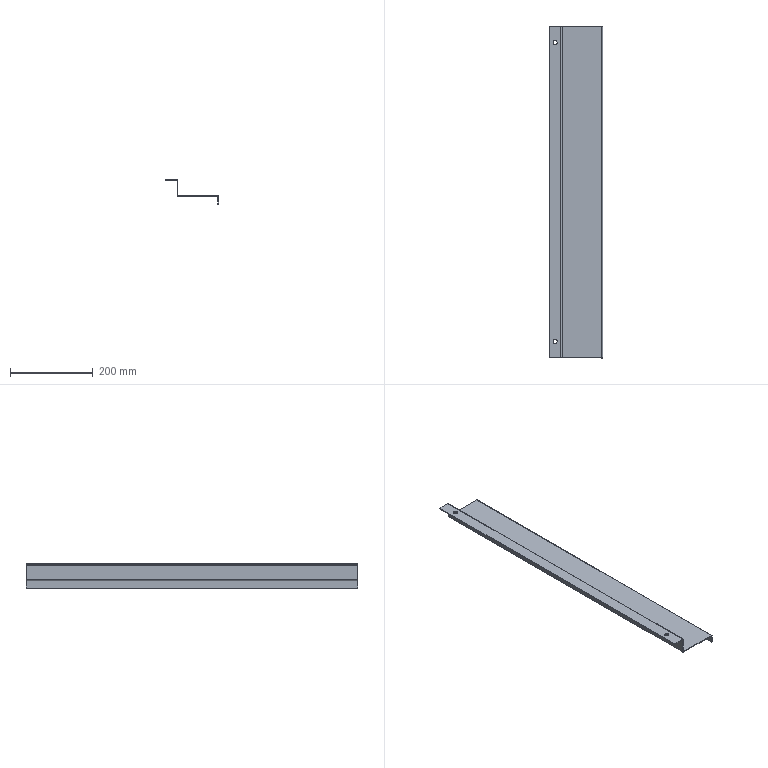Part | SolidWorks | features EdgeFlange 3, FlatPattern 1, ICE 1, SMBaseFlange 1, SheetMetal 1 | 1 solid | 34 faces | box 128 x 800 x 58 mm | volume 290508 mm3 | plane 24 | cylinder 10 | commonest cylinder face diameters 10 x4 1.473 x3 5.473 x3
STEP:
#1=CARTESIAN_POINT('',(-43.414,41.343,36.));
#2=VERTEX_POINT('',#1);
#3=CARTESIAN_POINT('',(-53.414,41.343,36.));
#4=VERTEX_POINT('',#3);
#5=CARTESIAN_POINT('',(-48.414,41.343,36.));
#6=DIRECTION('',(0.,0.,-1.));
#7=DIRECTION('',(-1.,0.,0.));
#8=AXIS2_PLACEMENT_3D('',#5,#6,#7);
#9=CIRCLE('',#8,5.);
#10=EDGE_CURVE('',#2,#4,#9,.T.);
#11=ORIENTED_EDGE('',*,*,#10,.T.);
#12=CARTESIAN_POINT('',(-53.414,41.343,38.));
#13=VERTEX_POINT('',#12);
#14=CARTESIAN_POINT('',(-53.414,41.343,28.));
#15=DIRECTION('',(0.,0.,1.));
#16=VECTOR('',#15,1000.);
#17=LINE('',#14,#16);
#18=EDGE_CURVE('',#4,#13,#17,.T.);
#19=ORIENTED_EDGE('',*,*,#18,.T.);
#20=CARTESIAN_POINT('',(-43.414,41.343,38.));
#21=VERTEX_POINT('',#20);
#22=CARTESIAN_POINT('',(-48.414,41.343,38.));
#23=DIRECTION('',(0.,0.,1.));
#24=DIRECTION('',(1.,0.,0.));
#25=AXIS2_PLACEMENT_3D('',#22,#23,#24);
#26=CIRCLE('',#25,5.);
#27=EDGE_CURVE('',#13,#21,#26,.T.);
#28=ORIENTED_EDGE('',*,*,#27,.T.);
#29=CARTESIAN_POINT('',(-43.414,41.343,28.));
#30=DIRECTION('',(0.,0.,1.));
#31=VECTOR('',#30,1000.);
#32=LINE('',#29,#31);
#33=EDGE_CURVE('',#2,#21,#32,.T.);
#34=ORIENTED_EDGE('',*,*,#33,.F.);
#35=EDGE_LOOP('',(#11,#19,#28,#34));
#36=FACE_OUTER_BOUND('',#35,.T.);
#37=CARTESIAN_POINT('',(-48.414,41.343,28.));
#38=DIRECTION('',(0.,0.,1.));
#39=DIRECTION('',(1.,0.,0.));
#40=AXIS2_PLACEMENT_3D('',#37,#38,#39);
#41=CYLINDRICAL_SURFACE('',#40,5.);
#42=ADVANCED_FACE('',(#36),#41,.F.);
#43=CARTESIAN_POINT('',(-43.414,-678.657,36.));
#44=VERTEX_POINT('',#43);
#45=CARTESIAN_POINT('',(-53.414,-678.657,36.));
#46=VERTEX_POINT('',#45);
#47=CARTESIAN_POINT('',(-48.414,-678.657,36.));
#48=DIRECTION('',(0.,0.,-1.));
#49=DIRECTION('',(-1.,0.,0.));
#50=AXIS2_PLACEMENT_3D('',#47,#48,#49);
#51=CIRCLE('',#50,5.);
#52=EDGE_CURVE('',#44,#46,#51,.T.);
#53=ORIENTED_EDGE('',*,*,#52,.T.);
#54=CARTESIAN_POINT('',(-53.414,-678.657,38.));
#55=VERTEX_POINT('',#54);
#56=CARTESIAN_POINT('',(-53.414,-678.657,28.));
#57=DIRECTION('',(0.,0.,1.));
#58=VECTOR('',#57,1000.);
#59=LINE('',#56,#58);
#60=EDGE_CURVE('',#46,#55,#59,.T.);
#61=ORIENTED_EDGE('',*,*,#60,.T.);
#62=CARTESIAN_POINT('',(-43.414,-678.657,38.));
#63=VERTEX_POINT('',#62);
#64=CARTESIAN_POINT('',(-48.414,-678.657,38.));
#65=DIRECTION('',(0.,0.,1.));
#66=DIRECTION('',(1.,0.,0.));
#67=AXIS2_PLACEMENT_3D('',#64,#65,#66);
#68=CIRCLE('',#67,5.);
#69=EDGE_CURVE('',#55,#63,#68,.T.);
#70=ORIENTED_EDGE('',*,*,#69,.T.);
#71=CARTESIAN_POINT('',(-43.414,-678.657,28.));
#72=DIRECTION('',(0.,0.,1.));
#73=VECTOR('',#72,1000.);
#74=LINE('',#71,#73);
#75=EDGE_CURVE('',#44,#63,#74,.T.);
#76=ORIENTED_EDGE('',*,*,#75,.F.);
#77=EDGE_LOOP('',(#53,#61,#70,#76));
#78=FACE_OUTER_BOUND('',#77,.T.);
#79=CARTESIAN_POINT('',(-48.414,-678.657,28.));
#80=DIRECTION('',(0.,0.,1.));
#81=DIRECTION('',(1.,0.,0.));
#82=AXIS2_PLACEMENT_3D('',#79,#80,#81);
#83=CYLINDRICAL_SURFACE('',#82,5.);
#84=ADVANCED_FACE('',(#78),#83,.F.);
#85=CARTESIAN_POINT('',(-34.046,-718.657,35.263));
#86=VERTEX_POINT('',#85);
#87=CARTESIAN_POINT('',(-32.046,-718.657,35.263));
#88=VERTEX_POINT('',#87);
#89=CARTESIAN_POINT('',(-34.046,-718.657,35.263));
#90=DIRECTION('',(1.,0.,0.));
#91=VECTOR('',#90,1000.);
#92=LINE('',#89,#91);
#93=EDGE_CURVE('',#86,#88,#92,.T.);
#94=ORIENTED_EDGE('',*,*,#93,.F.);
#95=CARTESIAN_POINT('',(-34.046,-718.657,0.7366));
#96=VERTEX_POINT('',#95);
#97=CARTESIAN_POINT('',(-34.046,-718.657,0.));
#98=DIRECTION('',(0.,0.,1.));
#99=VECTOR('',#98,1000.);
#100=LINE('',#97,#99);
#101=EDGE_CURVE('',#96,#86,#100,.T.);
#102=ORIENTED_EDGE('',*,*,#101,.F.);
#103=CARTESIAN_POINT('',(-32.046,-718.657,0.7366));
#104=VERTEX_POINT('',#103);
#105=CARTESIAN_POINT('',(-32.046,-718.657,0.7366));
#106=DIRECTION('',(-1.,0.,0.));
#107=VECTOR('',#106,1000.);
#108=LINE('',#105,#107);
#109=EDGE_CURVE('',#104,#96,#108,.T.);
#110=ORIENTED_EDGE('',*,*,#109,.F.);
#111=CARTESIAN_POINT('',(-32.046,-718.657,38.));
#112=DIRECTION('',(0.,0.,1.));
#113=VECTOR('',#112,1000.);
#114=LINE('',#111,#113);
#115=EDGE_CURVE('',#104,#88,#114,.T.);
#116=ORIENTED_EDGE('',*,*,#115,.T.);
#117=EDGE_LOOP('',(#94,#102,#110,#116));
#118=FACE_OUTER_BOUND('',#117,.T.);
#119=CARTESIAN_POINT('',(-34.046,-718.657,38.));
#120=DIRECTION('',(0.,1.,0.));
#121=DIRECTION('',(-1.,0.,0.));
#122=AXIS2_PLACEMENT_3D('',#119,#120,#121);
#123=PLANE('',#122);
#124=ADVANCED_FACE('',(#118),#123,.F.);
#125=CARTESIAN_POINT('',(-34.046,81.343,35.263));
#126=VERTEX_POINT('',#125);
#127=CARTESIAN_POINT('',(-32.046,81.343,35.263));
#128=VERTEX_POINT('',#127);
#129=CARTESIAN_POINT('',(-34.046,81.343,35.263));
#130=DIRECTION('',(1.,0.,0.));
#131=VECTOR('',#130,1000.);
#132=LINE('',#129,#131);
#133=EDGE_CURVE('',#126,#128,#132,.T.);
#134=ORIENTED_EDGE('',*,*,#133,.T.);
#135=CARTESIAN_POINT('',(-32.046,81.343,0.7366));
#136=VERTEX_POINT('',#135);
#137=CARTESIAN_POINT('',(-32.046,81.343,0.));
#138=DIRECTION('',(0.,0.,-1.));
#139=VECTOR('',#138,1000.);
#140=LINE('',#137,#139);
#141=EDGE_CURVE('',#128,#136,#140,.T.);
#142=ORIENTED_EDGE('',*,*,#141,.T.);
#143=CARTESIAN_POINT('',(-34.046,81.343,0.7366));
#144=VERTEX_POINT('',#143);
#145=CARTESIAN_POINT('',(-34.046,81.343,0.7366));
#146=DIRECTION('',(-1.,0.,0.));
#147=VECTOR('',#146,1000.);
#148=LINE('',#145,#147);
#149=EDGE_CURVE('',#136,#144,#148,.T.);
#150=ORIENTED_EDGE('',*,*,#149,.T.);
#151=CARTESIAN_POINT('',(-34.046,81.343,0.));
#152=DIRECTION('',(0.,0.,-1.));
#153=VECTOR('',#152,1000.);
#154=LINE('',#151,#153);
#155=EDGE_CURVE('',#126,#144,#154,.T.);
#156=ORIENTED_EDGE('',*,*,#155,.F.);
#157=EDGE_LOOP('',(#134,#142,#150,#156));
#158=FACE_OUTER_BOUND('',#157,.T.);
#159=CARTESIAN_POINT('',(-34.046,81.343,0.));
#160=DIRECTION('',(0.,-1.,0.));
#161=DIRECTION('',(0.,0.,-1.));
#162=AXIS2_PLACEMENT_3D('',#159,#160,#161);
#163=PLANE('',#162);
#164=ADVANCED_FACE('',(#158),#163,.F.);
#165=CARTESIAN_POINT('',(-34.046,81.343,35.263));
#166=DIRECTION('',(0.,-1.,0.));
#167=VECTOR('',#166,1000.);
#168=LINE('',#165,#167);
#169=EDGE_CURVE('',#126,#86,#168,.T.);
#170=ORIENTED_EDGE('',*,*,#169,.F.);
#171=ORIENTED_EDGE('',*,*,#155,.T.);
#172=CARTESIAN_POINT('',(-34.046,81.343,0.7366));
#173=DIRECTION('',(0.,1.,0.));
#174=VECTOR('',#173,1000.);
#175=LINE('',#172,#174);
#176=EDGE_CURVE('',#96,#144,#175,.T.);
#177=ORIENTED_EDGE('',*,*,#176,.F.);
#178=ORIENTED_EDGE('',*,*,#101,.T.);
#179=EDGE_LOOP('',(#170,#171,#177,#178));
#180=FACE_OUTER_BOUND('',#179,.T.);
#181=CARTESIAN_POINT('',(-34.046,0.,0.));
#182=DIRECTION('',(1.,0.,0.));
#183=DIRECTION('',(0.,0.,-1.));
#184=AXIS2_PLACEMENT_3D('',#181,#182,#183);
#185=PLANE('',#184);
#186=ADVANCED_FACE('',(#180),#185,.F.);
#187=ORIENTED_EDGE('',*,*,#141,.F.);
#188=CARTESIAN_POINT('',(-32.046,81.343,35.263));
#189=DIRECTION('',(0.,-1.,0.));
#190=VECTOR('',#189,1000.);
#191=LINE('',#188,#190);
#192=EDGE_CURVE('',#128,#88,#191,.T.);
#193=ORIENTED_EDGE('',*,*,#192,.T.);
#194=ORIENTED_EDGE('',*,*,#115,.F.);
#195=CARTESIAN_POINT('',(-32.046,81.343,0.7366));
#196=DIRECTION('',(0.,-1.,0.));
#197=VECTOR('',#196,1000.);
#198=LINE('',#195,#197);
#199=EDGE_CURVE('',#136,#104,#198,.T.);
#200=ORIENTED_EDGE('',*,*,#199,.F.);
#201=EDGE_LOOP('',(#187,#193,#194,#200));
#202=FACE_OUTER_BOUND('',#201,.T.);
#203=CARTESIAN_POINT('',(-32.046,0.,0.));
#204=DIRECTION('',(1.,0.,0.));
#205=DIRECTION('',(0.,0.,-1.));
#206=AXIS2_PLACEMENT_3D('',#203,#204,#205);
#207=PLANE('',#206);
#208=ADVANCED_FACE('',(#202),#207,.T.);
#209=CARTESIAN_POINT('',(-31.309,-718.657,-2.));
#210=VERTEX_POINT('',#209);
#211=CARTESIAN_POINT('',(63.218,-718.657,-2.));
#212=VERTEX_POINT('',#211);
#213=CARTESIAN_POINT('',(65.954,-718.657,-2.));
#214=DIRECTION('',(1.,0.,0.));
#215=VECTOR('',#214,1000.);
#216=LINE('',#213,#215);
#217=EDGE_CURVE('',#210,#212,#216,.T.);
#218=ORIENTED_EDGE('',*,*,#217,.T.);
#219=CARTESIAN_POINT('',(63.218,-718.657,0.));
#220=VERTEX_POINT('',#219);
#221=CARTESIAN_POINT('',(63.218,-718.657,-2.));
#222=DIRECTION('',(0.,0.,1.));
#223=VECTOR('',#222,1000.);
#224=LINE('',#221,#223);
#225=EDGE_CURVE('',#212,#220,#224,.T.);
#226=ORIENTED_EDGE('',*,*,#225,.T.);
#227=CARTESIAN_POINT('',(-31.309,-718.657,0.));
#228=VERTEX_POINT('',#227);
#229=CARTESIAN_POINT('',(65.954,-718.657,0.));
#230=DIRECTION('',(1.,0.,0.));
#231=VECTOR('',#230,1000.);
#232=LINE('',#229,#231);
#233=EDGE_CURVE('',#228,#220,#232,.T.);
#234=ORIENTED_EDGE('',*,*,#233,.F.);
#235=CARTESIAN_POINT('',(-31.309,-718.657,0.));
#236=DIRECTION('',(0.,0.,-1.));
#237=VECTOR('',#236,1000.);
#238=LINE('',#235,#237);
#239=EDGE_CURVE('',#228,#210,#238,.T.);
#240=ORIENTED_EDGE('',*,*,#239,.T.);
#241=EDGE_LOOP('',(#218,#226,#234,#240));
#242=FACE_OUTER_BOUND('',#241,.T.);
#243=CARTESIAN_POINT('',(65.954,-718.657,-2.));
#244=DIRECTION('',(0.,-1.,0.));
#245=DIRECTION('',(0.,0.,-1.));
#246=AXIS2_PLACEMENT_3D('',#243,#244,#245);
#247=PLANE('',#246);
#248=ADVANCED_FACE('',(#242),#247,.T.);
#249=CARTESIAN_POINT('',(63.218,81.343,-2.));
#250=VERTEX_POINT('',#249);
#251=CARTESIAN_POINT('',(-31.309,81.343,-2.));
#252=VERTEX_POINT('',#251);
#253=CARTESIAN_POINT('',(65.954,81.343,-2.));
#254=DIRECTION('',(-1.,0.,0.));
#255=VECTOR('',#254,1000.);
#256=LINE('',#253,#255);
#257=EDGE_CURVE('',#250,#252,#256,.T.);
#258=ORIENTED_EDGE('',*,*,#257,.F.);
#259=CARTESIAN_POINT('',(63.218,-718.657,-2.));
#260=DIRECTION('',(0.,1.,0.));
#261=VECTOR('',#260,1000.);
#262=LINE('',#259,#261);
#263=EDGE_CURVE('',#212,#250,#262,.T.);
#264=ORIENTED_EDGE('',*,*,#263,.F.);
#265=ORIENTED_EDGE('',*,*,#217,.F.);
#266=CARTESIAN_POINT('',(-31.309,-718.657,-2.));
#267=DIRECTION('',(0.,1.,0.));
#268=VECTOR('',#267,1000.);
#269=LINE('',#266,#268);
#270=EDGE_CURVE('',#210,#252,#269,.T.);
#271=ORIENTED_EDGE('',*,*,#270,.T.);
#272=EDGE_LOOP('',(#258,#264,#265,#271));
#273=FACE_OUTER_BOUND('',#272,.T.);
#274=CARTESIAN_POINT('',(0.,0.,-2.));
#275=DIRECTION('',(0.,0.,-1.));
#276=DIRECTION('',(-1.,0.,0.));
#277=AXIS2_PLACEMENT_3D('',#274,#275,#276);
#278=PLANE('',#277);
#279=ADVANCED_FACE('',(#273),#278,.T.);
#280=CARTESIAN_POINT('',(63.218,81.343,0.));
#281=VERTEX_POINT('',#280);
#282=CARTESIAN_POINT('',(63.218,-718.657,0.));
#283=DIRECTION('',(0.,1.,0.));
#284=VECTOR('',#283,1000.);
#285=LINE('',#282,#284);
#286=EDGE_CURVE('',#220,#281,#285,.T.);
#287=ORIENTED_EDGE('',*,*,#286,.T.);
#288=CARTESIAN_POINT('',(-31.309,81.343,0.));
#289=VERTEX_POINT('',#288);
#290=CARTESIAN_POINT('',(65.954,81.343,0.));
#291=DIRECTION('',(-1.,0.,0.));
#292=VECTOR('',#291,1000.);
#293=LINE('',#290,#292);
#294=EDGE_CURVE('',#281,#289,#293,.T.);
#295=ORIENTED_EDGE('',*,*,#294,.T.);
#296=CARTESIAN_POINT('',(-31.309,-718.657,0.));
#297=DIRECTION('',(0.,1.,0.));
#298=VECTOR('',#297,1000.);
#299=LINE('',#296,#298);
#300=EDGE_CURVE('',#228,#289,#299,.T.);
#301=ORIENTED_EDGE('',*,*,#300,.F.);
#302=ORIENTED_EDGE('',*,*,#233,.T.);
#303=EDGE_LOOP('',(#287,#295,#301,#302));
#304=FACE_OUTER_BOUND('',#303,.T.);
#305=CARTESIAN_POINT('',(0.,0.,0.));
#306=DIRECTION('',(0.,0.,-1.));
#307=DIRECTION('',(-1.,0.,0.));
#308=AXIS2_PLACEMENT_3D('',#305,#306,#307);
#309=PLANE('',#308);
#310=ADVANCED_FACE('',(#304),#309,.F.);
#311=CARTESIAN_POINT('',(63.218,81.343,-2.));
#312=DIRECTION('',(0.,0.,1.));
#313=VECTOR('',#312,1000.);
#314=LINE('',#311,#313);
#315=EDGE_CURVE('',#250,#281,#314,.T.);
#316=ORIENTED_EDGE('',*,*,#315,.F.);
#317=ORIENTED_EDGE('',*,*,#257,.T.);
#318=CARTESIAN_POINT('',(-31.309,81.343,0.));
#319=DIRECTION('',(0.,0.,-1.));
#320=VECTOR('',#319,1000.);
#321=LINE('',#318,#320);
#322=EDGE_CURVE('',#289,#252,#321,.T.);
#323=ORIENTED_EDGE('',*,*,#322,.F.);
#324=ORIENTED_EDGE('',*,*,#294,.F.);
#325=EDGE_LOOP('',(#316,#317,#323,#324));
#326=FACE_OUTER_BOUND('',#325,.T.);
#327=CARTESIAN_POINT('',(65.954,81.343,-2.));
#328=DIRECTION('',(0.,1.,0.));
#329=DIRECTION('',(-1.,0.,0.));
#330=AXIS2_PLACEMENT_3D('',#327,#328,#329);
#331=PLANE('',#330);
#332=ADVANCED_FACE('',(#326),#331,.T.);
#333=ORIENTED_EDGE('',*,*,#149,.F.);
#334=CARTESIAN_POINT('',(-31.309,81.343,0.7366));
#335=DIRECTION('',(0.,1.,0.));
#336=DIRECTION('',(0.,0.,-1.));
#337=AXIS2_PLACEMENT_3D('',#334,#335,#336);
#338=CIRCLE('',#337,0.7366);
#339=EDGE_CURVE('',#289,#136,#338,.T.);
#340=ORIENTED_EDGE('',*,*,#339,.F.);
#341=ORIENTED_EDGE('',*,*,#322,.T.);
#342=CARTESIAN_POINT('',(-31.309,81.343,0.7366));
#343=DIRECTION('',(0.,1.,0.));
#344=DIRECTION('',(0.,0.,-1.));
#345=AXIS2_PLACEMENT_3D('',#342,#343,#344);
#346=CIRCLE('',#345,2.737);
#347=EDGE_CURVE('',#252,#144,#346,.T.);
#348=ORIENTED_EDGE('',*,*,#347,.T.);
#349=EDGE_LOOP('',(#333,#340,#341,#348));
#350=FACE_OUTER_BOUND('',#349,.T.);
#351=CARTESIAN_POINT('',(-31.309,81.343,0.7366));
#352=DIRECTION('',(0.,1.,0.));
#353=DIRECTION('',(0.,0.,1.));
#354=AXIS2_PLACEMENT_3D('',#351,#352,#353);
#355=PLANE('',#354);
#356=ADVANCED_FACE('',(#350),#355,.T.);
#357=CARTESIAN_POINT('',(-31.309,-718.657,0.7366));
#358=DIRECTION('',(0.,-1.,0.));
#359=DIRECTION('',(0.,0.,-1.));
#360=AXIS2_PLACEMENT_3D('',#357,#358,#359);
#361=CIRCLE('',#360,0.7366);
#362=EDGE_CURVE('',#104,#228,#361,.T.);
#363=ORIENTED_EDGE('',*,*,#362,.F.);
#364=ORIENTED_EDGE('',*,*,#109,.T.);
#365=CARTESIAN_POINT('',(-31.309,-718.657,0.7366));
#366=DIRECTION('',(0.,-1.,0.));
#367=DIRECTION('',(0.,0.,-1.));
#368=AXIS2_PLACEMENT_3D('',#365,#366,#367);
#369=CIRCLE('',#368,2.737);
#370=EDGE_CURVE('',#96,#210,#369,.T.);
#371=ORIENTED_EDGE('',*,*,#370,.T.);
#372=ORIENTED_EDGE('',*,*,#239,.F.);
#373=EDGE_LOOP('',(#363,#364,#371,#372));
#374=FACE_OUTER_BOUND('',#373,.T.);
#375=CARTESIAN_POINT('',(-31.309,-718.657,0.7366));
#376=DIRECTION('',(0.,1.,0.));
#377=DIRECTION('',(0.,0.,1.));
#378=AXIS2_PLACEMENT_3D('',#375,#376,#377);
#379=PLANE('',#378);
#380=ADVANCED_FACE('',(#374),#379,.F.);
#381=ORIENTED_EDGE('',*,*,#270,.F.);
#382=ORIENTED_EDGE('',*,*,#370,.F.);
#383=ORIENTED_EDGE('',*,*,#176,.T.);
#384=ORIENTED_EDGE('',*,*,#347,.F.);
#385=EDGE_LOOP('',(#381,#382,#383,#384));
#386=FACE_OUTER_BOUND('',#385,.T.);
#387=CARTESIAN_POINT('',(-31.309,-718.657,0.7366));
#388=DIRECTION('',(0.,-1.,0.));
#389=DIRECTION('',(-1.,0.,0.));
#390=AXIS2_PLACEMENT_3D('',#387,#388,#389);
#391=CYLINDRICAL_SURFACE('',#390,2.737);
#392=ADVANCED_FACE('',(#386),#391,.T.);
#393=ORIENTED_EDGE('',*,*,#300,.T.);
#394=ORIENTED_EDGE('',*,*,#339,.T.);
#395=ORIENTED_EDGE('',*,*,#199,.T.);
#396=ORIENTED_EDGE('',*,*,#362,.T.);
#397=EDGE_LOOP('',(#393,#394,#395,#396));
#398=FACE_OUTER_BOUND('',#397,.T.);
#399=CARTESIAN_POINT('',(-31.309,-718.657,0.7366));
#400=DIRECTION('',(0.,-1.,0.));
#401=DIRECTION('',(-1.,0.,0.));
#402=AXIS2_PLACEMENT_3D('',#399,#400,#401);
#403=CYLINDRICAL_SURFACE('',#402,0.7366);
#404=ADVANCED_FACE('',(#398),#403,.F.);
#405=CARTESIAN_POINT('',(63.954,81.343,-2.737));
#406=VERTEX_POINT('',#405);
#407=CARTESIAN_POINT('',(65.954,81.343,-2.737));
#408=VERTEX_POINT('',#407);
#409=CARTESIAN_POINT('',(65.954,81.343,-2.737));
#410=DIRECTION('',(1.,0.,0.));
#411=VECTOR('',#410,1000.);
#412=LINE('',#409,#411);
#413=EDGE_CURVE('',#406,#408,#412,.T.);
#414=ORIENTED_EDGE('',*,*,#413,.F.);
#415=CARTESIAN_POINT('',(63.218,81.343,-2.737));
#416=DIRECTION('',(0.,1.,0.));
#417=DIRECTION('',(0.,0.,-1.));
#418=AXIS2_PLACEMENT_3D('',#415,#416,#417);
#419=CIRCLE('',#418,0.7366);
#420=EDGE_CURVE('',#250,#406,#419,.T.);
#421=ORIENTED_EDGE('',*,*,#420,.F.);
#422=ORIENTED_EDGE('',*,*,#315,.T.);
#423=CARTESIAN_POINT('',(63.218,81.343,-2.737));
#424=DIRECTION('',(0.,1.,0.));
#425=DIRECTION('',(0.,0.,-1.));
#426=AXIS2_PLACEMENT_3D('',#423,#424,#425);
#427=CIRCLE('',#426,2.737);
#428=EDGE_CURVE('',#281,#408,#427,.T.);
#429=ORIENTED_EDGE('',*,*,#428,.T.);
#430=EDGE_LOOP('',(#414,#421,#422,#429));
#431=FACE_OUTER_BOUND('',#430,.T.);
#432=CARTESIAN_POINT('',(63.218,81.343,-2.737));
#433=DIRECTION('',(0.,1.,0.));
#434=DIRECTION('',(0.,0.,1.));
#435=AXIS2_PLACEMENT_3D('',#432,#433,#434);
#436=PLANE('',#435);
#437=ADVANCED_FACE('',(#431),#436,.T.);
#438=CARTESIAN_POINT('',(63.954,-718.657,-2.737));
#439=VERTEX_POINT('',#438);
#440=CARTESIAN_POINT('',(63.218,-718.657,-2.737));
#441=DIRECTION('',(0.,-1.,0.));
#442=DIRECTION('',(0.,0.,-1.));
#443=AXIS2_PLACEMENT_3D('',#440,#441,#442);
#444=CIRCLE('',#443,0.7366);
#445=EDGE_CURVE('',#439,#212,#444,.T.);
#446=ORIENTED_EDGE('',*,*,#445,.F.);
#447=CARTESIAN_POINT('',(65.954,-718.657,-2.737));
#448=VERTEX_POINT('',#447);
#449=CARTESIAN_POINT('',(63.954,-718.657,-2.737));
#450=DIRECTION('',(1.,0.,0.));
#451=VECTOR('',#450,1000.);
#452=LINE('',#449,#451);
#453=EDGE_CURVE('',#439,#448,#452,.T.);
#454=ORIENTED_EDGE('',*,*,#453,.T.);
#455=CARTESIAN_POINT('',(63.218,-718.657,-2.737));
#456=DIRECTION('',(0.,-1.,0.));
#457=DIRECTION('',(0.,0.,-1.));
#458=AXIS2_PLACEMENT_3D('',#455,#456,#457);
#459=CIRCLE('',#458,2.737);
#460=EDGE_CURVE('',#448,#220,#459,.T.);
#461=ORIENTED_EDGE('',*,*,#460,.T.);
#462=ORIENTED_EDGE('',*,*,#225,.F.);
#463=EDGE_LOOP('',(#446,#454,#461,#462));
#464=FACE_OUTER_BOUND('',#463,.T.);
#465=CARTESIAN_POINT('',(63.218,-718.657,-2.737));
#466=DIRECTION('',(0.,1.,0.));
#467=DIRECTION('',(0.,0.,1.));
#468=AXIS2_PLACEMENT_3D('',#465,#466,#467);
#469=PLANE('',#468);
#470=ADVANCED_FACE('',(#464),#469,.F.);
#471=ORIENTED_EDGE('',*,*,#286,.F.);
#472=ORIENTED_EDGE('',*,*,#460,.F.);
#473=CARTESIAN_POINT('',(65.954,0.,-2.737));
#474=DIRECTION('',(0.,-1.,0.));
#475=VECTOR('',#474,1000.);
#476=LINE('',#473,#475);
#477=EDGE_CURVE('',#408,#448,#476,.T.);
#478=ORIENTED_EDGE('',*,*,#477,.F.);
#479=ORIENTED_EDGE('',*,*,#428,.F.);
#480=EDGE_LOOP('',(#471,#472,#478,#479));
#481=FACE_OUTER_BOUND('',#480,.T.);
#482=CARTESIAN_POINT('',(63.218,-718.657,-2.737));
#483=DIRECTION('',(0.,-1.,0.));
#484=DIRECTION('',(1.,0.,0.));
#485=AXIS2_PLACEMENT_3D('',#482,#483,#484);
#486=CYLINDRICAL_SURFACE('',#485,2.737);
#487=ADVANCED_FACE('',(#481),#486,.T.);
#488=ORIENTED_EDGE('',*,*,#263,.T.);
#489=ORIENTED_EDGE('',*,*,#420,.T.);
#490=CARTESIAN_POINT('',(63.954,81.343,-2.737));
#491=DIRECTION('',(0.,-1.,0.));
#492=VECTOR('',#491,1000.);
#493=LINE('',#490,#492);
#494=EDGE_CURVE('',#406,#439,#493,.T.);
#495=ORIENTED_EDGE('',*,*,#494,.T.);
#496=ORIENTED_EDGE('',*,*,#445,.T.);
#497=EDGE_LOOP('',(#488,#489,#495,#496));
#498=FACE_OUTER_BOUND('',#497,.T.);
#499=CARTESIAN_POINT('',(63.218,-718.657,-2.737));
#500=DIRECTION('',(0.,-1.,0.));
#501=DIRECTION('',(1.,0.,0.));
#502=AXIS2_PLACEMENT_3D('',#499,#500,#501);
#503=CYLINDRICAL_SURFACE('',#502,0.7366);
#504=ADVANCED_FACE('',(#498),#503,.F.);
#505=CARTESIAN_POINT('',(65.954,-718.657,-20.));
#506=VERTEX_POINT('',#505);
#507=CARTESIAN_POINT('',(65.954,-718.657,-2.));
#508=DIRECTION('',(0.,0.,1.));
#509=VECTOR('',#508,1000.);
#510=LINE('',#507,#509);
#511=EDGE_CURVE('',#506,#448,#510,.T.);
#512=ORIENTED_EDGE('',*,*,#511,.T.);
#513=ORIENTED_EDGE('',*,*,#453,.F.);
#514=CARTESIAN_POINT('',(63.954,-718.657,-20.));
#515=VERTEX_POINT('',#514);
#516=CARTESIAN_POINT('',(63.954,-718.657,0.));
#517=DIRECTION('',(0.,0.,1.));
#518=VECTOR('',#517,1000.);
#519=LINE('',#516,#518);
#520=EDGE_CURVE('',#515,#439,#519,.T.);
#521=ORIENTED_EDGE('',*,*,#520,.F.);
#522=CARTESIAN_POINT('',(65.954,-718.657,-20.));
#523=DIRECTION('',(-1.,0.,0.));
#524=VECTOR('',#523,1000.);
#525=LINE('',#522,#524);
#526=EDGE_CURVE('',#506,#515,#525,.T.);
#527=ORIENTED_EDGE('',*,*,#526,.F.);
#528=EDGE_LOOP('',(#512,#513,#521,#527));
#529=FACE_OUTER_BOUND('',#528,.T.);
#530=CARTESIAN_POINT('',(65.954,-718.657,-2.));
#531=DIRECTION('',(0.,-1.,0.));
#532=DIRECTION('',(1.,0.,0.));
#533=AXIS2_PLACEMENT_3D('',#530,#531,#532);
#534=PLANE('',#533);
#535=ADVANCED_FACE('',(#529),#534,.T.);
#536=CARTESIAN_POINT('',(63.954,81.343,-20.));
#537=VERTEX_POINT('',#536);
#538=CARTESIAN_POINT('',(63.954,81.343,0.));
#539=DIRECTION('',(0.,0.,-1.));
#540=VECTOR('',#539,1000.);
#541=LINE('',#538,#540);
#542=EDGE_CURVE('',#406,#537,#541,.T.);
#543=ORIENTED_EDGE('',*,*,#542,.F.);
#544=ORIENTED_EDGE('',*,*,#413,.T.);
#545=CARTESIAN_POINT('',(65.954,81.343,-20.));
#546=VERTEX_POINT('',#545);
#547=CARTESIAN_POINT('',(65.954,81.343,-20.));
#548=DIRECTION('',(0.,0.,-1.));
#549=VECTOR('',#548,1000.);
#550=LINE('',#547,#549);
#551=EDGE_CURVE('',#408,#546,#550,.T.);
#552=ORIENTED_EDGE('',*,*,#551,.T.);
#553=CARTESIAN_POINT('',(65.954,81.343,-20.));
#554=DIRECTION('',(-1.,0.,0.));
#555=VECTOR('',#554,1000.);
#556=LINE('',#553,#555);
#557=EDGE_CURVE('',#546,#537,#556,.T.);
#558=ORIENTED_EDGE('',*,*,#557,.T.);
#559=EDGE_LOOP('',(#543,#544,#552,#558));
#560=FACE_OUTER_BOUND('',#559,.T.);
#561=CARTESIAN_POINT('',(65.954,81.343,-20.));
#562=DIRECTION('',(0.,1.,0.));
#563=DIRECTION('',(-1.,0.,0.));
#564=AXIS2_PLACEMENT_3D('',#561,#562,#563);
#565=PLANE('',#564);
#566=ADVANCED_FACE('',(#560),#565,.T.);
#567=ORIENTED_EDGE('',*,*,#551,.F.);
#568=ORIENTED_EDGE('',*,*,#477,.T.);
#569=ORIENTED_EDGE('',*,*,#511,.F.);
#570=CARTESIAN_POINT('',(65.954,-718.657,-20.));
#571=DIRECTION('',(0.,-1.,0.));
#572=VECTOR('',#571,1000.);
#573=LINE('',#570,#572);
#574=EDGE_CURVE('',#546,#506,#573,.T.);
#575=ORIENTED_EDGE('',*,*,#574,.F.);
#576=EDGE_LOOP('',(#567,#568,#569,#575));
#577=FACE_OUTER_BOUND('',#576,.T.);
#578=CARTESIAN_POINT('',(65.954,0.,0.));
#579=DIRECTION('',(1.,0.,0.));
#580=DIRECTION('',(0.,0.,-1.));
#581=AXIS2_PLACEMENT_3D('',#578,#579,#580);
#582=PLANE('',#581);
#583=ADVANCED_FACE('',(#577),#582,.T.);
#584=ORIENTED_EDGE('',*,*,#494,.F.);
#585=ORIENTED_EDGE('',*,*,#542,.T.);
#586=CARTESIAN_POINT('',(63.954,0.,-20.));
#587=DIRECTION('',(0.,-1.,0.));
#588=VECTOR('',#587,1000.);
#589=LINE('',#586,#588);
#590=EDGE_CURVE('',#537,#515,#589,.T.);
#591=ORIENTED_EDGE('',*,*,#590,.T.);
#592=ORIENTED_EDGE('',*,*,#520,.T.);
#593=EDGE_LOOP('',(#584,#585,#591,#592));
#594=FACE_OUTER_BOUND('',#593,.T.);
#595=CARTESIAN_POINT('',(63.954,0.,0.));
#596=DIRECTION('',(1.,0.,0.));
#597=DIRECTION('',(0.,0.,-1.));
#598=AXIS2_PLACEMENT_3D('',#595,#596,#597);
#599=PLANE('',#598);
#600=ADVANCED_FACE('',(#594),#599,.F.);
#601=ORIENTED_EDGE('',*,*,#590,.F.);
#602=ORIENTED_EDGE('',*,*,#557,.F.);
#603=ORIENTED_EDGE('',*,*,#574,.T.);
#604=ORIENTED_EDGE('',*,*,#526,.T.);
#605=EDGE_LOOP('',(#601,#602,#603,#604));
#606=FACE_OUTER_BOUND('',#605,.T.);
#607=CARTESIAN_POINT('',(65.954,-718.657,-20.));
#608=DIRECTION('',(0.,0.,-1.));
#609=DIRECTION('',(-1.,0.,0.));
#610=AXIS2_PLACEMENT_3D('',#607,#608,#609);
#611=PLANE('',#610);
#612=ADVANCED_FACE('',(#606),#611,.T.);
#613=CARTESIAN_POINT('',(-34.782,-718.657,36.));
#614=VERTEX_POINT('',#613);
#615=CARTESIAN_POINT('',(-34.782,-718.657,38.));
#616=VERTEX_POINT('',#615);
#617=CARTESIAN_POINT('',(-34.782,-718.657,38.));
#618=DIRECTION('',(0.,0.,1.));
#619=VECTOR('',#618,1000.);
#620=LINE('',#617,#619);
#621=EDGE_CURVE('',#614,#616,#620,.T.);
#622=ORIENTED_EDGE('',*,*,#621,.F.);
#623=CARTESIAN_POINT('',(-34.782,-718.657,35.263));
#624=DIRECTION('',(0.,-1.,0.));
#625=DIRECTION('',(0.,0.,1.));
#626=AXIS2_PLACEMENT_3D('',#623,#624,#625);
#627=CIRCLE('',#626,0.7366);
#628=EDGE_CURVE('',#86,#614,#627,.T.);
#629=ORIENTED_EDGE('',*,*,#628,.F.);
#630=ORIENTED_EDGE('',*,*,#93,.T.);
#631=CARTESIAN_POINT('',(-34.782,-718.657,35.263));
#632=DIRECTION('',(0.,-1.,0.));
#633=DIRECTION('',(0.,0.,1.));
#634=AXIS2_PLACEMENT_3D('',#631,#632,#633);
#635=CIRCLE('',#634,2.737);
#636=EDGE_CURVE('',#88,#616,#635,.T.);
#637=ORIENTED_EDGE('',*,*,#636,.T.);
#638=EDGE_LOOP('',(#622,#629,#630,#637));
#639=FACE_OUTER_BOUND('',#638,.T.);
#640=CARTESIAN_POINT('',(-34.782,-718.657,35.263));
#641=DIRECTION('',(0.,-1.,0.));
#642=DIRECTION('',(0.,0.,-1.));
#643=AXIS2_PLACEMENT_3D('',#640,#641,#642);
#644=PLANE('',#643);
#645=ADVANCED_FACE('',(#639),#644,.T.);
#646=CARTESIAN_POINT('',(-34.782,81.343,36.));
#647=VERTEX_POINT('',#646);
#648=CARTESIAN_POINT('',(-34.782,81.343,35.263));
#649=DIRECTION('',(0.,1.,0.));
#650=DIRECTION('',(0.,0.,1.));
#651=AXIS2_PLACEMENT_3D('',#648,#649,#650);
#652=CIRCLE('',#651,0.7366);
#653=EDGE_CURVE('',#647,#126,#652,.T.);
#654=ORIENTED_EDGE('',*,*,#653,.F.);
#655=CARTESIAN_POINT('',(-34.782,81.343,38.));
#656=VERTEX_POINT('',#655);
#657=CARTESIAN_POINT('',(-34.782,81.343,36.));
#658=DIRECTION('',(0.,0.,1.));
#659=VECTOR('',#658,1000.);
#660=LINE('',#657,#659);
#661=EDGE_CURVE('',#647,#656,#660,.T.);
#662=ORIENTED_EDGE('',*,*,#661,.T.);
#663=CARTESIAN_POINT('',(-34.782,81.343,35.263));
#664=DIRECTION('',(0.,1.,0.));
#665=DIRECTION('',(0.,0.,1.));
#666=AXIS2_PLACEMENT_3D('',#663,#664,#665);
#667=CIRCLE('',#666,2.737);
#668=EDGE_CURVE('',#656,#128,#667,.T.);
#669=ORIENTED_EDGE('',*,*,#668,.T.);
#670=ORIENTED_EDGE('',*,*,#133,.F.);
#671=EDGE_LOOP('',(#654,#662,#669,#670));
#672=FACE_OUTER_BOUND('',#671,.T.);
#673=CARTESIAN_POINT('',(-34.782,81.343,35.263));
#674=DIRECTION('',(0.,-1.,0.));
#675=DIRECTION('',(0.,0.,-1.));
#676=AXIS2_PLACEMENT_3D('',#673,#674,#675);
#677=PLANE('',#676);
#678=ADVANCED_FACE('',(#672),#677,.F.);
#679=ORIENTED_EDGE('',*,*,#192,.F.);
#680=ORIENTED_EDGE('',*,*,#668,.F.);
#681=CARTESIAN_POINT('',(-34.782,-718.657,38.));
#682=DIRECTION('',(0.,-1.,0.));
#683=VECTOR('',#682,1000.);
#684=LINE('',#681,#683);
#685=EDGE_CURVE('',#656,#616,#684,.T.);
#686=ORIENTED_EDGE('',*,*,#685,.T.);
#687=ORIENTED_EDGE('',*,*,#636,.F.);
#688=EDGE_LOOP('',(#679,#680,#686,#687));
#689=FACE_OUTER_BOUND('',#688,.T.);
#690=CARTESIAN_POINT('',(-34.782,81.343,35.263));
#691=DIRECTION('',(0.,1.,0.));
#692=DIRECTION('',(0.,0.,1.));
#693=AXIS2_PLACEMENT_3D('',#690,#691,#692);
#694=CYLINDRICAL_SURFACE('',#693,2.737);
#695=ADVANCED_FACE('',(#689),#694,.T.);
#696=ORIENTED_EDGE('',*,*,#169,.T.);
#697=ORIENTED_EDGE('',*,*,#628,.T.);
#698=CARTESIAN_POINT('',(-34.782,-718.657,36.));
#699=DIRECTION('',(0.,1.,0.));
#700=VECTOR('',#699,1000.);
#701=LINE('',#698,#700);
#702=EDGE_CURVE('',#614,#647,#701,.T.);
#703=ORIENTED_EDGE('',*,*,#702,.T.);
#704=ORIENTED_EDGE('',*,*,#653,.T.);
#705=EDGE_LOOP('',(#696,#697,#703,#704));
#706=FACE_OUTER_BOUND('',#705,.T.);
#707=CARTESIAN_POINT('',(-34.782,81.343,35.263));
#708=DIRECTION('',(0.,1.,0.));
#709=DIRECTION('',(0.,0.,1.));
#710=AXIS2_PLACEMENT_3D('',#707,#708,#709);
#711=CYLINDRICAL_SURFACE('',#710,0.7366);
#712=ADVANCED_FACE('',(#706),#711,.F.);
#713=ORIENTED_EDGE('',*,*,#621,.T.);
#714=CARTESIAN_POINT('',(-62.046,-718.657,38.));
#715=VERTEX_POINT('',#714);
#716=CARTESIAN_POINT('',(0.,-718.657,38.));
#717=DIRECTION('',(1.,0.,0.));
#718=VECTOR('',#717,1000.);
#719=LINE('',#716,#718);
#720=EDGE_CURVE('',#715,#616,#719,.T.);
#721=ORIENTED_EDGE('',*,*,#720,.F.);
#722=CARTESIAN_POINT('',(-62.046,-718.657,36.));
#723=VERTEX_POINT('',#722);
#724=CARTESIAN_POINT('',(-62.046,-718.657,38.));
#725=DIRECTION('',(0.,0.,-1.));
#726=VECTOR('',#725,1000.);
#727=LINE('',#724,#726);
#728=EDGE_CURVE('',#715,#723,#727,.T.);
#729=ORIENTED_EDGE('',*,*,#728,.T.);
#730=CARTESIAN_POINT('',(-34.046,-718.657,36.));
#731=DIRECTION('',(1.,0.,0.));
#732=VECTOR('',#731,1000.);
#733=LINE('',#730,#732);
#734=EDGE_CURVE('',#723,#614,#733,.T.);
#735=ORIENTED_EDGE('',*,*,#734,.T.);
#736=EDGE_LOOP('',(#713,#721,#729,#735));
#737=FACE_OUTER_BOUND('',#736,.T.);
#738=CARTESIAN_POINT('',(-34.046,-718.657,38.));
#739=DIRECTION('',(0.,1.,0.));
#740=DIRECTION('',(0.,0.,1.));
#741=AXIS2_PLACEMENT_3D('',#738,#739,#740);
#742=PLANE('',#741);
#743=ADVANCED_FACE('',(#737),#742,.F.);
#744=ORIENTED_EDGE('',*,*,#661,.F.);
#745=CARTESIAN_POINT('',(-62.046,81.343,36.));
#746=VERTEX_POINT('',#745);
#747=CARTESIAN_POINT('',(-62.046,81.343,36.));
#748=DIRECTION('',(-1.,0.,0.));
#749=VECTOR('',#748,1000.);
#750=LINE('',#747,#749);
#751=EDGE_CURVE('',#647,#746,#750,.T.);
#752=ORIENTED_EDGE('',*,*,#751,.T.);
#753=CARTESIAN_POINT('',(-62.046,81.343,38.));
#754=VERTEX_POINT('',#753);
#755=CARTESIAN_POINT('',(-62.046,81.343,38.));
#756=DIRECTION('',(0.,0.,-1.));
#757=VECTOR('',#756,1000.);
#758=LINE('',#755,#757);
#759=EDGE_CURVE('',#754,#746,#758,.T.);
#760=ORIENTED_EDGE('',*,*,#759,.F.);
#761=CARTESIAN_POINT('',(0.,81.343,38.));
#762=DIRECTION('',(-1.,0.,0.));
#763=VECTOR('',#762,1000.);
#764=LINE('',#761,#763);
#765=EDGE_CURVE('',#656,#754,#764,.T.);
#766=ORIENTED_EDGE('',*,*,#765,.F.);
#767=EDGE_LOOP('',(#744,#752,#760,#766));
#768=FACE_OUTER_BOUND('',#767,.T.);
#769=CARTESIAN_POINT('',(-62.046,81.343,38.));
#770=DIRECTION('',(0.,-1.,0.));
#771=DIRECTION('',(0.,0.,-1.));
#772=AXIS2_PLACEMENT_3D('',#769,#770,#771);
#773=PLANE('',#772);
#774=ADVANCED_FACE('',(#768),#773,.F.);
#775=CARTESIAN_POINT('',(-48.414,41.343,38.));
#776=DIRECTION('',(0.,0.,1.));
#777=DIRECTION('',(1.,0.,0.));
#778=AXIS2_PLACEMENT_3D('',#775,#776,#777);
#779=CIRCLE('',#778,5.);
#780=EDGE_CURVE('',#21,#13,#779,.T.);
#781=ORIENTED_EDGE('',*,*,#780,.F.);
#782=ORIENTED_EDGE('',*,*,#27,.F.);
#783=EDGE_LOOP('',(#781,#782));
#784=FACE_BOUND('',#783,.T.);
#785=CARTESIAN_POINT('',(-48.414,-678.657,38.));
#786=DIRECTION('',(0.,0.,1.));
#787=DIRECTION('',(1.,0.,0.));
#788=AXIS2_PLACEMENT_3D('',#785,#786,#787);
#789=CIRCLE('',#788,5.);
#790=EDGE_CURVE('',#63,#55,#789,.T.);
#791=ORIENTED_EDGE('',*,*,#790,.F.);
#792=ORIENTED_EDGE('',*,*,#69,.F.);
#793=EDGE_LOOP('',(#791,#792));
#794=FACE_BOUND('',#793,.T.);
#795=ORIENTED_EDGE('',*,*,#685,.F.);
#796=ORIENTED_EDGE('',*,*,#765,.T.);
#797=CARTESIAN_POINT('',(-62.046,0.,38.));
#798=DIRECTION('',(0.,-1.,0.));
#799=VECTOR('',#798,1000.);
#800=LINE('',#797,#799);
#801=EDGE_CURVE('',#754,#715,#800,.T.);
#802=ORIENTED_EDGE('',*,*,#801,.T.);
#803=ORIENTED_EDGE('',*,*,#720,.T.);
#804=EDGE_LOOP('',(#795,#796,#802,#803));
#805=FACE_OUTER_BOUND('',#804,.T.);
#806=CARTESIAN_POINT('',(0.,0.,38.));
#807=DIRECTION('',(0.,0.,-1.));
#808=DIRECTION('',(-1.,0.,0.));
#809=AXIS2_PLACEMENT_3D('',#806,#807,#808);
#810=PLANE('',#809);
#811=ADVANCED_FACE('',(#784,#794,#805),#810,.F.);
#812=ORIENTED_EDGE('',*,*,#10,.F.);
#813=CARTESIAN_POINT('',(-48.414,41.343,36.));
#814=DIRECTION('',(0.,0.,-1.));
#815=DIRECTION('',(-1.,0.,0.));
#816=AXIS2_PLACEMENT_3D('',#813,#814,#815);
#817=CIRCLE('',#816,5.);
#818=EDGE_CURVE('',#4,#2,#817,.T.);
#819=ORIENTED_EDGE('',*,*,#818,.F.);
#820=EDGE_LOOP('',(#812,#819));
#821=FACE_BOUND('',#820,.T.);
#822=ORIENTED_EDGE('',*,*,#52,.F.);
#823=CARTESIAN_POINT('',(-48.414,-678.657,36.));
#824=DIRECTION('',(0.,0.,-1.));
#825=DIRECTION('',(-1.,0.,0.));
#826=AXIS2_PLACEMENT_3D('',#823,#824,#825);
#827=CIRCLE('',#826,5.);
#828=EDGE_CURVE('',#46,#44,#827,.T.);
#829=ORIENTED_EDGE('',*,*,#828,.F.);
#830=EDGE_LOOP('',(#822,#829));
#831=FACE_BOUND('',#830,.T.);
#832=ORIENTED_EDGE('',*,*,#751,.F.);
#833=ORIENTED_EDGE('',*,*,#702,.F.);
#834=ORIENTED_EDGE('',*,*,#734,.F.);
#835=CARTESIAN_POINT('',(-62.046,-718.657,36.));
#836=DIRECTION('',(0.,-1.,0.));
#837=VECTOR('',#836,1000.);
#838=LINE('',#835,#837);
#839=EDGE_CURVE('',#746,#723,#838,.T.);
#840=ORIENTED_EDGE('',*,*,#839,.F.);
#841=EDGE_LOOP('',(#832,#833,#834,#840));
#842=FACE_OUTER_BOUND('',#841,.T.);
#843=CARTESIAN_POINT('',(0.,0.,36.));
#844=DIRECTION('',(0.,0.,-1.));
#845=DIRECTION('',(-1.,0.,0.));
#846=AXIS2_PLACEMENT_3D('',#843,#844,#845);
#847=PLANE('',#846);
#848=ADVANCED_FACE('',(#821,#831,#842),#847,.T.);
#849=ORIENTED_EDGE('',*,*,#839,.T.);
#850=ORIENTED_EDGE('',*,*,#728,.F.);
#851=ORIENTED_EDGE('',*,*,#801,.F.);
#852=ORIENTED_EDGE('',*,*,#759,.T.);
#853=EDGE_LOOP('',(#849,#850,#851,#852));
#854=FACE_OUTER_BOUND('',#853,.T.);
#855=CARTESIAN_POINT('',(-62.046,-718.657,38.));
#856=DIRECTION('',(1.,0.,0.));
#857=DIRECTION('',(0.,1.,0.));
#858=AXIS2_PLACEMENT_3D('',#855,#856,#857);
#859=PLANE('',#858);
#860=ADVANCED_FACE('',(#854),#859,.F.);
#861=ORIENTED_EDGE('',*,*,#60,.F.);
#862=ORIENTED_EDGE('',*,*,#828,.T.);
#863=ORIENTED_EDGE('',*,*,#75,.T.);
#864=ORIENTED_EDGE('',*,*,#790,.T.);
#865=EDGE_LOOP('',(#861,#862,#863,#864));
#866=FACE_OUTER_BOUND('',#865,.T.);
#867=CARTESIAN_POINT('',(-48.414,-678.657,28.));
#868=DIRECTION('',(0.,0.,1.));
#869=DIRECTION('',(1.,0.,0.));
#870=AXIS2_PLACEMENT_3D('',#867,#868,#869);
#871=CYLINDRICAL_SURFACE('',#870,5.);
#872=ADVANCED_FACE('',(#866),#871,.F.);
#873=ORIENTED_EDGE('',*,*,#18,.F.);
#874=ORIENTED_EDGE('',*,*,#818,.T.);
#875=ORIENTED_EDGE('',*,*,#33,.T.);
#876=ORIENTED_EDGE('',*,*,#780,.T.);
#877=EDGE_LOOP('',(#873,#874,#875,#876));
#878=FACE_OUTER_BOUND('',#877,.T.);
#879=CARTESIAN_POINT('',(-48.414,41.343,28.));
#880=DIRECTION('',(0.,0.,1.));
#881=DIRECTION('',(1.,0.,0.));
#882=AXIS2_PLACEMENT_3D('',#879,#880,#881);
#883=CYLINDRICAL_SURFACE('',#882,5.);
#884=ADVANCED_FACE('',(#878),#883,.F.);
#885=CLOSED_SHELL('',(#42,#84,#124,#164,#186,#208,#248,#279,#310,#332,#356,#380,#392,#404,#437,#470,#487,#504,#535,#566,#583,#600,#612,#645,#678,#695,#712,#743,#774,#811,#848,#860,#872,#884));
#886=MANIFOLD_SOLID_BREP('',#885);
#887=CARTESIAN_POINT('',(0.,0.,0.));
#888=DIRECTION('',(0.,0.,1.));
#889=DIRECTION('',(1.,0.,0.));
#890=AXIS2_PLACEMENT_3D('',#887,#888,#889);
#891=(LENGTH_UNIT()NAMED_UNIT(*)SI_UNIT(.MILLI.,.METRE.));
#892=UNCERTAINTY_MEASURE_WITH_UNIT(LENGTH_MEASURE(0.00001),#891,'','');
#893=(NAMED_UNIT(*)PLANE_ANGLE_UNIT()SI_UNIT($,.RADIAN.));
#894=(NAMED_UNIT(*)SI_UNIT($,.STERADIAN.)SOLID_ANGLE_UNIT());
#895=(GEOMETRIC_REPRESENTATION_CONTEXT(3)GLOBAL_UNCERTAINTY_ASSIGNED_CONTEXT((#892))GLOBAL_UNIT_ASSIGNED_CONTEXT((#891,#893,#894))REPRESENTATION_CONTEXT('',''));
#896=ADVANCED_BREP_SHAPE_REPRESENTATION('',(#886,#890),#895);